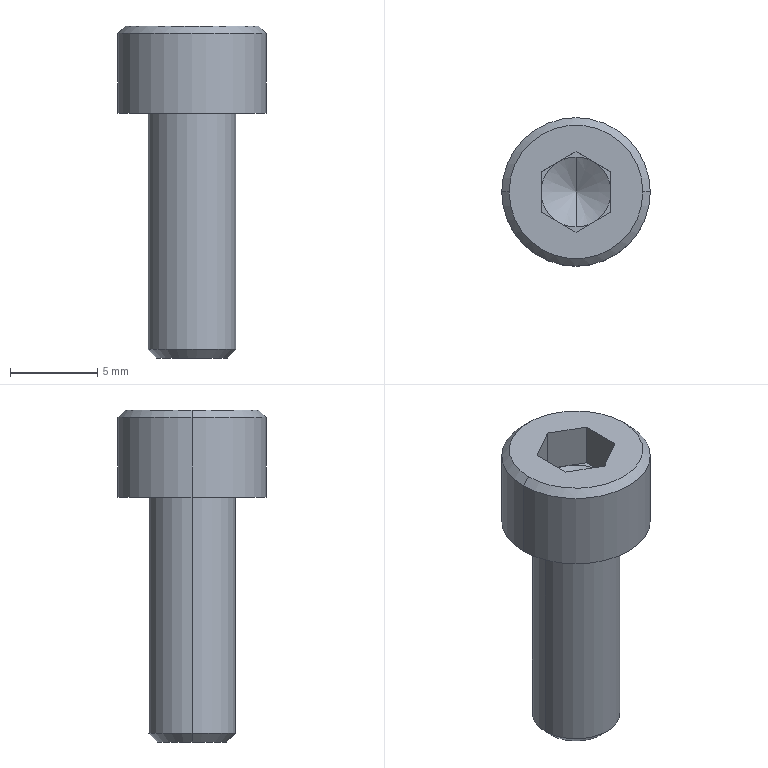Part | NX | features BREP 1 | 1 solid | 25 faces | box 8.5 x 8.5 x 19 mm | volume 515.039 mm3 | plane 15 | cone 6 | cylinder 4 | commonest cylinder face diameters 5 x2 8.5 x2
STEP:
#1=CARTESIAN_POINT('',(0.,-2.,2.5));
#2=VERTEX_POINT('',#1);
#3=CARTESIAN_POINT('',(0.,0.,1.345));
#4=VERTEX_POINT('',#3);
#5=CARTESIAN_POINT('',(0.,0.,1.345));
#6=DIRECTION('',(0.,-0.866,0.5));
#7=VECTOR('',#6,1000.);
#8=LINE('',#5,#7);
#9=EDGE_CURVE('',#2,#4,#8,.F.);
#10=ORIENTED_EDGE('',*,*,#9,.T.);
#11=CARTESIAN_POINT('',(0.,2.,2.5));
#12=VERTEX_POINT('',#11);
#13=CARTESIAN_POINT('',(0.,0.,1.345));
#14=DIRECTION('',(0.,0.866,0.5));
#15=VECTOR('',#14,1000.);
#16=LINE('',#13,#15);
#17=EDGE_CURVE('',#12,#4,#16,.F.);
#18=ORIENTED_EDGE('',*,*,#17,.F.);
#19=CARTESIAN_POINT('',(-1.,1.732,2.5));
#20=VERTEX_POINT('',#19);
#21=CARTESIAN_POINT('',(0.,0.,2.5));
#22=DIRECTION('',(0.,0.,1.));
#23=DIRECTION('',(0.,-1.,0.));
#24=AXIS2_PLACEMENT_3D('',#21,#22,#23);
#25=CIRCLE('',#24,2.);
#26=EDGE_CURVE('',#12,#20,#25,.T.);
#27=ORIENTED_EDGE('',*,*,#26,.T.);
#28=CARTESIAN_POINT('',(-2.,0.,2.5));
#29=VERTEX_POINT('',#28);
#30=CARTESIAN_POINT('',(0.,0.,2.5));
#31=DIRECTION('',(0.,0.,1.));
#32=DIRECTION('',(0.,-1.,0.));
#33=AXIS2_PLACEMENT_3D('',#30,#31,#32);
#34=CIRCLE('',#33,2.);
#35=EDGE_CURVE('',#20,#29,#34,.T.);
#36=ORIENTED_EDGE('',*,*,#35,.T.);
#37=CARTESIAN_POINT('',(-1.,-1.732,2.5));
#38=VERTEX_POINT('',#37);
#39=CARTESIAN_POINT('',(0.,0.,2.5));
#40=DIRECTION('',(0.,0.,1.));
#41=DIRECTION('',(0.,-1.,0.));
#42=AXIS2_PLACEMENT_3D('',#39,#40,#41);
#43=CIRCLE('',#42,2.);
#44=EDGE_CURVE('',#29,#38,#43,.T.);
#45=ORIENTED_EDGE('',*,*,#44,.T.);
#46=CARTESIAN_POINT('',(0.,0.,2.5));
#47=DIRECTION('',(0.,0.,1.));
#48=DIRECTION('',(0.,-1.,0.));
#49=AXIS2_PLACEMENT_3D('',#46,#47,#48);
#50=CIRCLE('',#49,2.);
#51=EDGE_CURVE('',#38,#2,#50,.T.);
#52=ORIENTED_EDGE('',*,*,#51,.T.);
#53=EDGE_LOOP('',(#10,#18,#27,#36,#45,#52));
#54=FACE_BOUND('',#53,.T.);
#55=CARTESIAN_POINT('',(0.,0.,1001.345));
#56=DIRECTION('',(0.,0.,1.));
#57=DIRECTION('',(0.,1.,0.));
#58=AXIS2_PLACEMENT_3D('',#55,#56,#57);
#59=CONICAL_SURFACE('',#58,1732.051,1.047);
#60=ADVANCED_FACE('',(#54),#59,.F.);
#61=CARTESIAN_POINT('',(4.25,0.,0.));
#62=VERTEX_POINT('',#61);
#63=CARTESIAN_POINT('',(-4.25,0.,0.));
#64=VERTEX_POINT('',#63);
#65=CARTESIAN_POINT('',(0.,0.,0.));
#66=DIRECTION('',(0.,0.,1.));
#67=DIRECTION('',(1.,0.,0.));
#68=AXIS2_PLACEMENT_3D('',#65,#66,#67);
#69=CIRCLE('',#68,4.25);
#70=EDGE_CURVE('',#62,#64,#69,.T.);
#71=ORIENTED_EDGE('',*,*,#70,.T.);
#72=CARTESIAN_POINT('',(-4.25,0.,4.575));
#73=VERTEX_POINT('',#72);
#74=CARTESIAN_POINT('',(-4.25,0.,0.));
#75=DIRECTION('',(0.,0.,1.));
#76=VECTOR('',#75,1000.);
#77=LINE('',#74,#76);
#78=EDGE_CURVE('',#64,#73,#77,.T.);
#79=ORIENTED_EDGE('',*,*,#78,.T.);
#80=CARTESIAN_POINT('',(4.25,0.,4.575));
#81=VERTEX_POINT('',#80);
#82=CARTESIAN_POINT('',(0.,0.,4.575));
#83=DIRECTION('',(0.,0.,1.));
#84=DIRECTION('',(1.,0.,0.));
#85=AXIS2_PLACEMENT_3D('',#82,#83,#84);
#86=CIRCLE('',#85,4.25);
#87=EDGE_CURVE('',#81,#73,#86,.T.);
#88=ORIENTED_EDGE('',*,*,#87,.F.);
#89=CARTESIAN_POINT('',(4.25,0.,0.));
#90=DIRECTION('',(0.,0.,1.));
#91=VECTOR('',#90,1000.);
#92=LINE('',#89,#91);
#93=EDGE_CURVE('',#62,#81,#92,.T.);
#94=ORIENTED_EDGE('',*,*,#93,.F.);
#95=EDGE_LOOP('',(#71,#79,#88,#94));
#96=FACE_BOUND('',#95,.T.);
#97=CARTESIAN_POINT('',(0.,0.,0.));
#98=DIRECTION('',(0.,0.,1.));
#99=DIRECTION('',(-1.,0.,0.));
#100=AXIS2_PLACEMENT_3D('',#97,#98,#99);
#101=CYLINDRICAL_SURFACE('',#100,4.25);
#102=ADVANCED_FACE('',(#96),#101,.T.);
#103=CARTESIAN_POINT('',(3.825,0.,5.));
#104=VERTEX_POINT('',#103);
#105=CARTESIAN_POINT('',(-3.825,0.,5.));
#106=VERTEX_POINT('',#105);
#107=CARTESIAN_POINT('',(0.,0.,5.));
#108=DIRECTION('',(0.,0.,1.));
#109=DIRECTION('',(1.,0.,0.));
#110=AXIS2_PLACEMENT_3D('',#107,#108,#109);
#111=CIRCLE('',#110,3.825);
#112=EDGE_CURVE('',#104,#106,#111,.T.);
#113=ORIENTED_EDGE('',*,*,#112,.F.);
#114=CARTESIAN_POINT('',(4.25,0.,4.575));
#115=DIRECTION('',(0.7071,0.,-0.7071));
#116=VECTOR('',#115,1000.);
#117=LINE('',#114,#116);
#118=EDGE_CURVE('',#81,#104,#117,.F.);
#119=ORIENTED_EDGE('',*,*,#118,.F.);
#120=ORIENTED_EDGE('',*,*,#87,.T.);
#121=CARTESIAN_POINT('',(-4.25,0.,4.575));
#122=DIRECTION('',(-0.7071,0.,-0.7071));
#123=VECTOR('',#122,1000.);
#124=LINE('',#121,#123);
#125=EDGE_CURVE('',#73,#106,#124,.F.);
#126=ORIENTED_EDGE('',*,*,#125,.T.);
#127=EDGE_LOOP('',(#113,#119,#120,#126));
#128=FACE_BOUND('',#127,.T.);
#129=CARTESIAN_POINT('',(0.,0.,4.575));
#130=DIRECTION('',(0.,0.,-1.));
#131=DIRECTION('',(1.,0.,0.));
#132=AXIS2_PLACEMENT_3D('',#129,#130,#131);
#133=CONICAL_SURFACE('',#132,4.25,0.7854);
#134=ADVANCED_FACE('',(#128),#133,.T.);
#135=CARTESIAN_POINT('',(2.01,0.,-14.));
#136=VERTEX_POINT('',#135);
#137=CARTESIAN_POINT('',(-2.01,0.,-14.));
#138=VERTEX_POINT('',#137);
#139=CARTESIAN_POINT('',(0.,0.,-14.));
#140=DIRECTION('',(0.,0.,1.));
#141=DIRECTION('',(1.,0.,0.));
#142=AXIS2_PLACEMENT_3D('',#139,#140,#141);
#143=CIRCLE('',#142,2.01);
#144=EDGE_CURVE('',#136,#138,#143,.T.);
#145=ORIENTED_EDGE('',*,*,#144,.T.);
#146=CARTESIAN_POINT('',(-2.5,0.,-13.509));
#147=VERTEX_POINT('',#146);
#148=CARTESIAN_POINT('',(-2.01,0.,-14.));
#149=DIRECTION('',(-0.7071,0.,0.7071));
#150=VECTOR('',#149,1000.);
#151=LINE('',#148,#150);
#152=EDGE_CURVE('',#138,#147,#151,.T.);
#153=ORIENTED_EDGE('',*,*,#152,.T.);
#154=CARTESIAN_POINT('',(2.5,0.,-13.509));
#155=VERTEX_POINT('',#154);
#156=CARTESIAN_POINT('',(0.,0.,-13.509));
#157=DIRECTION('',(0.,0.,1.));
#158=DIRECTION('',(1.,0.,0.));
#159=AXIS2_PLACEMENT_3D('',#156,#157,#158);
#160=CIRCLE('',#159,2.5);
#161=EDGE_CURVE('',#155,#147,#160,.T.);
#162=ORIENTED_EDGE('',*,*,#161,.F.);
#163=CARTESIAN_POINT('',(2.01,0.,-14.));
#164=DIRECTION('',(0.7071,0.,0.7071));
#165=VECTOR('',#164,1000.);
#166=LINE('',#163,#165);
#167=EDGE_CURVE('',#136,#155,#166,.T.);
#168=ORIENTED_EDGE('',*,*,#167,.F.);
#169=EDGE_LOOP('',(#145,#153,#162,#168));
#170=FACE_BOUND('',#169,.T.);
#171=CARTESIAN_POINT('',(0.,0.,-14.));
#172=DIRECTION('',(0.,0.,1.));
#173=DIRECTION('',(-1.,0.,0.));
#174=AXIS2_PLACEMENT_3D('',#171,#172,#173);
#175=CONICAL_SURFACE('',#174,2.01,0.7854);
#176=ADVANCED_FACE('',(#170),#175,.T.);
#177=ORIENTED_EDGE('',*,*,#161,.T.);
#178=CARTESIAN_POINT('',(-2.5,0.,0.));
#179=VERTEX_POINT('',#178);
#180=CARTESIAN_POINT('',(-2.5,0.,-14.));
#181=DIRECTION('',(0.,0.,1.));
#182=VECTOR('',#181,1000.);
#183=LINE('',#180,#182);
#184=EDGE_CURVE('',#147,#179,#183,.T.);
#185=ORIENTED_EDGE('',*,*,#184,.T.);
#186=CARTESIAN_POINT('',(2.5,0.,0.));
#187=VERTEX_POINT('',#186);
#188=CARTESIAN_POINT('',(0.,0.,0.));
#189=DIRECTION('',(0.,0.,1.));
#190=DIRECTION('',(1.,0.,0.));
#191=AXIS2_PLACEMENT_3D('',#188,#189,#190);
#192=CIRCLE('',#191,2.5);
#193=EDGE_CURVE('',#187,#179,#192,.T.);
#194=ORIENTED_EDGE('',*,*,#193,.F.);
#195=CARTESIAN_POINT('',(2.5,0.,-14.));
#196=DIRECTION('',(0.,0.,1.));
#197=VECTOR('',#196,1000.);
#198=LINE('',#195,#197);
#199=EDGE_CURVE('',#155,#187,#198,.T.);
#200=ORIENTED_EDGE('',*,*,#199,.F.);
#201=EDGE_LOOP('',(#177,#185,#194,#200));
#202=FACE_BOUND('',#201,.T.);
#203=CARTESIAN_POINT('',(0.,0.,-14.));
#204=DIRECTION('',(0.,0.,1.));
#205=DIRECTION('',(-1.,0.,0.));
#206=AXIS2_PLACEMENT_3D('',#203,#204,#205);
#207=CYLINDRICAL_SURFACE('',#206,2.5);
#208=ADVANCED_FACE('',(#202),#207,.T.);
#209=CARTESIAN_POINT('',(1.,-1.732,2.5));
#210=VERTEX_POINT('',#209);
#211=CARTESIAN_POINT('',(2.,0.,2.5));
#212=VERTEX_POINT('',#211);
#213=CARTESIAN_POINT('',(0.,0.,2.5));
#214=DIRECTION('',(0.,0.,1.));
#215=DIRECTION('',(0.,-1.,0.));
#216=AXIS2_PLACEMENT_3D('',#213,#214,#215);
#217=CIRCLE('',#216,2.);
#218=EDGE_CURVE('',#210,#212,#217,.T.);
#219=ORIENTED_EDGE('',*,*,#218,.F.);
#220=CARTESIAN_POINT('',(2.,-1.155,2.5));
#221=VERTEX_POINT('',#220);
#222=CARTESIAN_POINT('',(0.,-2.309,2.5));
#223=DIRECTION('',(0.866,0.5,0.));
#224=VECTOR('',#223,1000.);
#225=LINE('',#222,#224);
#226=EDGE_CURVE('',#210,#221,#225,.T.);
#227=ORIENTED_EDGE('',*,*,#226,.T.);
#228=CARTESIAN_POINT('',(2.,-1.155,2.5));
#229=DIRECTION('',(0.,1.,0.));
#230=VECTOR('',#229,1000.);
#231=LINE('',#228,#230);
#232=EDGE_CURVE('',#221,#212,#231,.T.);
#233=ORIENTED_EDGE('',*,*,#232,.T.);
#234=EDGE_LOOP('',(#219,#227,#233));
#235=FACE_BOUND('',#234,.T.);
#236=CARTESIAN_POINT('',(0.,0.,2.5));
#237=DIRECTION('',(0.,0.,1.));
#238=DIRECTION('',(-1.,0.,0.));
#239=AXIS2_PLACEMENT_3D('',#236,#237,#238);
#240=PLANE('',#239);
#241=ADVANCED_FACE('',(#235),#240,.T.);
#242=CARTESIAN_POINT('',(1.,1.732,2.5));
#243=VERTEX_POINT('',#242);
#244=CARTESIAN_POINT('',(0.,0.,2.5));
#245=DIRECTION('',(0.,0.,1.));
#246=DIRECTION('',(0.,-1.,0.));
#247=AXIS2_PLACEMENT_3D('',#244,#245,#246);
#248=CIRCLE('',#247,2.);
#249=EDGE_CURVE('',#212,#243,#248,.T.);
#250=ORIENTED_EDGE('',*,*,#249,.F.);
#251=CARTESIAN_POINT('',(2.,1.155,2.5));
#252=VERTEX_POINT('',#251);
#253=CARTESIAN_POINT('',(2.,-1.155,2.5));
#254=DIRECTION('',(0.,1.,0.));
#255=VECTOR('',#254,1000.);
#256=LINE('',#253,#255);
#257=EDGE_CURVE('',#212,#252,#256,.T.);
#258=ORIENTED_EDGE('',*,*,#257,.T.);
#259=CARTESIAN_POINT('',(2.,1.155,2.5));
#260=DIRECTION('',(-0.866,0.5,0.));
#261=VECTOR('',#260,1000.);
#262=LINE('',#259,#261);
#263=EDGE_CURVE('',#252,#243,#262,.T.);
#264=ORIENTED_EDGE('',*,*,#263,.T.);
#265=EDGE_LOOP('',(#250,#258,#264));
#266=FACE_BOUND('',#265,.T.);
#267=CARTESIAN_POINT('',(0.,0.,2.5));
#268=DIRECTION('',(0.,0.,1.));
#269=DIRECTION('',(-1.,0.,0.));
#270=AXIS2_PLACEMENT_3D('',#267,#268,#269);
#271=PLANE('',#270);
#272=ADVANCED_FACE('',(#266),#271,.T.);
#273=CARTESIAN_POINT('',(0.,0.,2.5));
#274=DIRECTION('',(0.,0.,1.));
#275=DIRECTION('',(0.,-1.,0.));
#276=AXIS2_PLACEMENT_3D('',#273,#274,#275);
#277=CIRCLE('',#276,2.);
#278=EDGE_CURVE('',#243,#12,#277,.T.);
#279=ORIENTED_EDGE('',*,*,#278,.F.);
#280=CARTESIAN_POINT('',(0.,2.309,2.5));
#281=VERTEX_POINT('',#280);
#282=CARTESIAN_POINT('',(2.,1.155,2.5));
#283=DIRECTION('',(-0.866,0.5,0.));
#284=VECTOR('',#283,1000.);
#285=LINE('',#282,#284);
#286=EDGE_CURVE('',#243,#281,#285,.T.);
#287=ORIENTED_EDGE('',*,*,#286,.T.);
#288=CARTESIAN_POINT('',(0.,2.309,2.5));
#289=DIRECTION('',(-0.866,-0.5,0.));
#290=VECTOR('',#289,1000.);
#291=LINE('',#288,#290);
#292=EDGE_CURVE('',#281,#20,#291,.T.);
#293=ORIENTED_EDGE('',*,*,#292,.T.);
#294=ORIENTED_EDGE('',*,*,#26,.F.);
#295=EDGE_LOOP('',(#279,#287,#293,#294));
#296=FACE_BOUND('',#295,.T.);
#297=CARTESIAN_POINT('',(0.,0.,2.5));
#298=DIRECTION('',(0.,0.,1.));
#299=DIRECTION('',(-1.,0.,0.));
#300=AXIS2_PLACEMENT_3D('',#297,#298,#299);
#301=PLANE('',#300);
#302=ADVANCED_FACE('',(#296),#301,.T.);
#303=ORIENTED_EDGE('',*,*,#35,.F.);
#304=CARTESIAN_POINT('',(-2.,1.155,2.5));
#305=VERTEX_POINT('',#304);
#306=CARTESIAN_POINT('',(0.,2.309,2.5));
#307=DIRECTION('',(-0.866,-0.5,0.));
#308=VECTOR('',#307,1000.);
#309=LINE('',#306,#308);
#310=EDGE_CURVE('',#20,#305,#309,.T.);
#311=ORIENTED_EDGE('',*,*,#310,.T.);
#312=CARTESIAN_POINT('',(-2.,1.155,2.5));
#313=DIRECTION('',(0.,-1.,0.));
#314=VECTOR('',#313,1000.);
#315=LINE('',#312,#314);
#316=EDGE_CURVE('',#305,#29,#315,.T.);
#317=ORIENTED_EDGE('',*,*,#316,.T.);
#318=EDGE_LOOP('',(#303,#311,#317));
#319=FACE_BOUND('',#318,.T.);
#320=CARTESIAN_POINT('',(0.,0.,2.5));
#321=DIRECTION('',(0.,0.,1.));
#322=DIRECTION('',(-1.,0.,0.));
#323=AXIS2_PLACEMENT_3D('',#320,#321,#322);
#324=PLANE('',#323);
#325=ADVANCED_FACE('',(#319),#324,.T.);
#326=ORIENTED_EDGE('',*,*,#44,.F.);
#327=CARTESIAN_POINT('',(-2.,-1.155,2.5));
#328=VERTEX_POINT('',#327);
#329=CARTESIAN_POINT('',(-2.,1.155,2.5));
#330=DIRECTION('',(0.,-1.,0.));
#331=VECTOR('',#330,1000.);
#332=LINE('',#329,#331);
#333=EDGE_CURVE('',#29,#328,#332,.T.);
#334=ORIENTED_EDGE('',*,*,#333,.T.);
#335=CARTESIAN_POINT('',(-2.,-1.155,2.5));
#336=DIRECTION('',(0.866,-0.5,0.));
#337=VECTOR('',#336,1000.);
#338=LINE('',#335,#337);
#339=EDGE_CURVE('',#328,#38,#338,.T.);
#340=ORIENTED_EDGE('',*,*,#339,.T.);
#341=EDGE_LOOP('',(#326,#334,#340));
#342=FACE_BOUND('',#341,.T.);
#343=CARTESIAN_POINT('',(0.,0.,2.5));
#344=DIRECTION('',(0.,0.,1.));
#345=DIRECTION('',(-1.,0.,0.));
#346=AXIS2_PLACEMENT_3D('',#343,#344,#345);
#347=PLANE('',#346);
#348=ADVANCED_FACE('',(#342),#347,.T.);
#349=ORIENTED_EDGE('',*,*,#184,.F.);
#350=CARTESIAN_POINT('',(0.,0.,-13.509));
#351=DIRECTION('',(0.,0.,1.));
#352=DIRECTION('',(1.,0.,0.));
#353=AXIS2_PLACEMENT_3D('',#350,#351,#352);
#354=CIRCLE('',#353,2.5);
#355=EDGE_CURVE('',#147,#155,#354,.T.);
#356=ORIENTED_EDGE('',*,*,#355,.T.);
#357=ORIENTED_EDGE('',*,*,#199,.T.);
#358=CARTESIAN_POINT('',(0.,0.,0.));
#359=DIRECTION('',(0.,0.,1.));
#360=DIRECTION('',(1.,0.,0.));
#361=AXIS2_PLACEMENT_3D('',#358,#359,#360);
#362=CIRCLE('',#361,2.5);
#363=EDGE_CURVE('',#179,#187,#362,.T.);
#364=ORIENTED_EDGE('',*,*,#363,.F.);
#365=EDGE_LOOP('',(#349,#356,#357,#364));
#366=FACE_BOUND('',#365,.T.);
#367=CARTESIAN_POINT('',(0.,0.,-14.));
#368=DIRECTION('',(0.,0.,1.));
#369=DIRECTION('',(-1.,0.,0.));
#370=AXIS2_PLACEMENT_3D('',#367,#368,#369);
#371=CYLINDRICAL_SURFACE('',#370,2.5);
#372=ADVANCED_FACE('',(#366),#371,.T.);
#373=ORIENTED_EDGE('',*,*,#152,.F.);
#374=CARTESIAN_POINT('',(0.,0.,-14.));
#375=DIRECTION('',(0.,0.,1.));
#376=DIRECTION('',(1.,0.,0.));
#377=AXIS2_PLACEMENT_3D('',#374,#375,#376);
#378=CIRCLE('',#377,2.01);
#379=EDGE_CURVE('',#138,#136,#378,.T.);
#380=ORIENTED_EDGE('',*,*,#379,.T.);
#381=ORIENTED_EDGE('',*,*,#167,.T.);
#382=ORIENTED_EDGE('',*,*,#355,.F.);
#383=EDGE_LOOP('',(#373,#380,#381,#382));
#384=FACE_BOUND('',#383,.T.);
#385=CARTESIAN_POINT('',(0.,0.,-14.));
#386=DIRECTION('',(0.,0.,1.));
#387=DIRECTION('',(-1.,0.,0.));
#388=AXIS2_PLACEMENT_3D('',#385,#386,#387);
#389=CONICAL_SURFACE('',#388,2.01,0.7854);
#390=ADVANCED_FACE('',(#384),#389,.T.);
#391=ORIENTED_EDGE('',*,*,#144,.F.);
#392=ORIENTED_EDGE('',*,*,#379,.F.);
#393=EDGE_LOOP('',(#391,#392));
#394=FACE_BOUND('',#393,.T.);
#395=CARTESIAN_POINT('',(0.,2.01,-14.));
#396=DIRECTION('',(0.,0.,1.));
#397=DIRECTION('',(-1.,0.,0.));
#398=AXIS2_PLACEMENT_3D('',#395,#396,#397);
#399=PLANE('',#398);
#400=ADVANCED_FACE('',(#394),#399,.F.);
#401=CARTESIAN_POINT('',(0.,-2.309,5.));
#402=VERTEX_POINT('',#401);
#403=CARTESIAN_POINT('',(2.,-1.155,5.));
#404=VERTEX_POINT('',#403);
#405=CARTESIAN_POINT('',(0.,-2.309,5.));
#406=DIRECTION('',(0.866,0.5,0.));
#407=VECTOR('',#406,1000.);
#408=LINE('',#405,#407);
#409=EDGE_CURVE('',#402,#404,#408,.T.);
#410=ORIENTED_EDGE('',*,*,#409,.F.);
#411=CARTESIAN_POINT('',(-2.,-1.155,5.));
#412=VERTEX_POINT('',#411);
#413=CARTESIAN_POINT('',(-2.,-1.155,5.));
#414=DIRECTION('',(0.866,-0.5,0.));
#415=VECTOR('',#414,1000.);
#416=LINE('',#413,#415);
#417=EDGE_CURVE('',#412,#402,#416,.T.);
#418=ORIENTED_EDGE('',*,*,#417,.F.);
#419=CARTESIAN_POINT('',(-2.,1.155,5.));
#420=VERTEX_POINT('',#419);
#421=CARTESIAN_POINT('',(-2.,1.155,5.));
#422=DIRECTION('',(0.,-1.,0.));
#423=VECTOR('',#422,1000.);
#424=LINE('',#421,#423);
#425=EDGE_CURVE('',#420,#412,#424,.T.);
#426=ORIENTED_EDGE('',*,*,#425,.F.);
#427=CARTESIAN_POINT('',(0.,2.309,5.));
#428=VERTEX_POINT('',#427);
#429=CARTESIAN_POINT('',(0.,2.309,5.));
#430=DIRECTION('',(-0.866,-0.5,0.));
#431=VECTOR('',#430,1000.);
#432=LINE('',#429,#431);
#433=EDGE_CURVE('',#428,#420,#432,.T.);
#434=ORIENTED_EDGE('',*,*,#433,.F.);
#435=CARTESIAN_POINT('',(2.,1.155,5.));
#436=VERTEX_POINT('',#435);
#437=CARTESIAN_POINT('',(2.,1.155,5.));
#438=DIRECTION('',(-0.866,0.5,0.));
#439=VECTOR('',#438,1000.);
#440=LINE('',#437,#439);
#441=EDGE_CURVE('',#436,#428,#440,.T.);
#442=ORIENTED_EDGE('',*,*,#441,.F.);
#443=CARTESIAN_POINT('',(2.,-1.155,5.));
#444=DIRECTION('',(0.,1.,0.));
#445=VECTOR('',#444,1000.);
#446=LINE('',#443,#445);
#447=EDGE_CURVE('',#404,#436,#446,.T.);
#448=ORIENTED_EDGE('',*,*,#447,.F.);
#449=EDGE_LOOP('',(#410,#418,#426,#434,#442,#448));
#450=FACE_BOUND('',#449,.T.);
#451=CARTESIAN_POINT('',(0.,0.,5.));
#452=DIRECTION('',(0.,0.,1.));
#453=DIRECTION('',(1.,0.,0.));
#454=AXIS2_PLACEMENT_3D('',#451,#452,#453);
#455=CIRCLE('',#454,3.825);
#456=EDGE_CURVE('',#106,#104,#455,.T.);
#457=ORIENTED_EDGE('',*,*,#456,.T.);
#458=ORIENTED_EDGE('',*,*,#112,.T.);
#459=EDGE_LOOP('',(#457,#458));
#460=FACE_BOUND('',#459,.T.);
#461=CARTESIAN_POINT('',(0.,0.,5.));
#462=DIRECTION('',(0.,0.,-1.));
#463=DIRECTION('',(1.,0.,0.));
#464=AXIS2_PLACEMENT_3D('',#461,#462,#463);
#465=PLANE('',#464);
#466=ADVANCED_FACE('',(#450,#460),#465,.F.);
#467=ORIENTED_EDGE('',*,*,#118,.T.);
#468=ORIENTED_EDGE('',*,*,#456,.F.);
#469=ORIENTED_EDGE('',*,*,#125,.F.);
#470=CARTESIAN_POINT('',(0.,0.,4.575));
#471=DIRECTION('',(0.,0.,1.));
#472=DIRECTION('',(1.,0.,0.));
#473=AXIS2_PLACEMENT_3D('',#470,#471,#472);
#474=CIRCLE('',#473,4.25);
#475=EDGE_CURVE('',#73,#81,#474,.T.);
#476=ORIENTED_EDGE('',*,*,#475,.T.);
#477=EDGE_LOOP('',(#467,#468,#469,#476));
#478=FACE_BOUND('',#477,.T.);
#479=CARTESIAN_POINT('',(0.,0.,4.575));
#480=DIRECTION('',(0.,0.,-1.));
#481=DIRECTION('',(1.,0.,0.));
#482=AXIS2_PLACEMENT_3D('',#479,#480,#481);
#483=CONICAL_SURFACE('',#482,4.25,0.7854);
#484=ADVANCED_FACE('',(#478),#483,.T.);
#485=ORIENTED_EDGE('',*,*,#78,.F.);
#486=CARTESIAN_POINT('',(0.,0.,0.));
#487=DIRECTION('',(0.,0.,1.));
#488=DIRECTION('',(1.,0.,0.));
#489=AXIS2_PLACEMENT_3D('',#486,#487,#488);
#490=CIRCLE('',#489,4.25);
#491=EDGE_CURVE('',#64,#62,#490,.T.);
#492=ORIENTED_EDGE('',*,*,#491,.T.);
#493=ORIENTED_EDGE('',*,*,#93,.T.);
#494=ORIENTED_EDGE('',*,*,#475,.F.);
#495=EDGE_LOOP('',(#485,#492,#493,#494));
#496=FACE_BOUND('',#495,.T.);
#497=CARTESIAN_POINT('',(0.,0.,0.));
#498=DIRECTION('',(0.,0.,1.));
#499=DIRECTION('',(-1.,0.,0.));
#500=AXIS2_PLACEMENT_3D('',#497,#498,#499);
#501=CYLINDRICAL_SURFACE('',#500,4.25);
#502=ADVANCED_FACE('',(#496),#501,.T.);
#503=ORIENTED_EDGE('',*,*,#193,.T.);
#504=ORIENTED_EDGE('',*,*,#363,.T.);
#505=EDGE_LOOP('',(#503,#504));
#506=FACE_BOUND('',#505,.T.);
#507=ORIENTED_EDGE('',*,*,#70,.F.);
#508=ORIENTED_EDGE('',*,*,#491,.F.);
#509=EDGE_LOOP('',(#507,#508));
#510=FACE_BOUND('',#509,.T.);
#511=CARTESIAN_POINT('',(0.,4.25,0.));
#512=DIRECTION('',(0.,0.,1.));
#513=DIRECTION('',(-1.,0.,0.));
#514=AXIS2_PLACEMENT_3D('',#511,#512,#513);
#515=PLANE('',#514);
#516=ADVANCED_FACE('',(#506,#510),#515,.F.);
#517=ORIENTED_EDGE('',*,*,#417,.T.);
#518=CARTESIAN_POINT('',(0.,-2.309,2.5));
#519=VERTEX_POINT('',#518);
#520=CARTESIAN_POINT('',(0.,-2.309,2.5));
#521=DIRECTION('',(0.,0.,1.));
#522=VECTOR('',#521,1000.);
#523=LINE('',#520,#522);
#524=EDGE_CURVE('',#519,#402,#523,.T.);
#525=ORIENTED_EDGE('',*,*,#524,.F.);
#526=CARTESIAN_POINT('',(-2.,-1.155,2.5));
#527=DIRECTION('',(0.866,-0.5,0.));
#528=VECTOR('',#527,1000.);
#529=LINE('',#526,#528);
#530=EDGE_CURVE('',#38,#519,#529,.T.);
#531=ORIENTED_EDGE('',*,*,#530,.F.);
#532=ORIENTED_EDGE('',*,*,#339,.F.);
#533=CARTESIAN_POINT('',(-2.,-1.155,2.5));
#534=DIRECTION('',(0.,0.,1.));
#535=VECTOR('',#534,1000.);
#536=LINE('',#533,#535);
#537=EDGE_CURVE('',#328,#412,#536,.T.);
#538=ORIENTED_EDGE('',*,*,#537,.T.);
#539=EDGE_LOOP('',(#517,#525,#531,#532,#538));
#540=FACE_BOUND('',#539,.T.);
#541=CARTESIAN_POINT('',(-2.,-1.155,2.5));
#542=DIRECTION('',(-0.5,-0.866,0.));
#543=DIRECTION('',(-0.866,0.5,0.));
#544=AXIS2_PLACEMENT_3D('',#541,#542,#543);
#545=PLANE('',#544);
#546=ADVANCED_FACE('',(#540),#545,.F.);
#547=ORIENTED_EDGE('',*,*,#425,.T.);
#548=ORIENTED_EDGE('',*,*,#537,.F.);
#549=ORIENTED_EDGE('',*,*,#333,.F.);
#550=ORIENTED_EDGE('',*,*,#316,.F.);
#551=CARTESIAN_POINT('',(-2.,1.155,2.5));
#552=DIRECTION('',(0.,0.,1.));
#553=VECTOR('',#552,1000.);
#554=LINE('',#551,#553);
#555=EDGE_CURVE('',#305,#420,#554,.T.);
#556=ORIENTED_EDGE('',*,*,#555,.T.);
#557=EDGE_LOOP('',(#547,#548,#549,#550,#556));
#558=FACE_BOUND('',#557,.T.);
#559=CARTESIAN_POINT('',(-2.,1.155,2.5));
#560=DIRECTION('',(-1.,0.,0.));
#561=DIRECTION('',(0.,0.,-1.));
#562=AXIS2_PLACEMENT_3D('',#559,#560,#561);
#563=PLANE('',#562);
#564=ADVANCED_FACE('',(#558),#563,.F.);
#565=ORIENTED_EDGE('',*,*,#433,.T.);
#566=ORIENTED_EDGE('',*,*,#555,.F.);
#567=ORIENTED_EDGE('',*,*,#310,.F.);
#568=ORIENTED_EDGE('',*,*,#292,.F.);
#569=CARTESIAN_POINT('',(0.,2.309,2.5));
#570=DIRECTION('',(0.,0.,1.));
#571=VECTOR('',#570,1000.);
#572=LINE('',#569,#571);
#573=EDGE_CURVE('',#281,#428,#572,.T.);
#574=ORIENTED_EDGE('',*,*,#573,.T.);
#575=EDGE_LOOP('',(#565,#566,#567,#568,#574));
#576=FACE_BOUND('',#575,.T.);
#577=CARTESIAN_POINT('',(0.,2.309,2.5));
#578=DIRECTION('',(-0.5,0.866,0.));
#579=DIRECTION('',(0.866,0.5,0.));
#580=AXIS2_PLACEMENT_3D('',#577,#578,#579);
#581=PLANE('',#580);
#582=ADVANCED_FACE('',(#576),#581,.F.);
#583=ORIENTED_EDGE('',*,*,#441,.T.);
#584=ORIENTED_EDGE('',*,*,#573,.F.);
#585=ORIENTED_EDGE('',*,*,#286,.F.);
#586=ORIENTED_EDGE('',*,*,#263,.F.);
#587=CARTESIAN_POINT('',(2.,1.155,2.5));
#588=DIRECTION('',(0.,0.,1.));
#589=VECTOR('',#588,1000.);
#590=LINE('',#587,#589);
#591=EDGE_CURVE('',#252,#436,#590,.T.);
#592=ORIENTED_EDGE('',*,*,#591,.T.);
#593=EDGE_LOOP('',(#583,#584,#585,#586,#592));
#594=FACE_BOUND('',#593,.T.);
#595=CARTESIAN_POINT('',(2.,1.155,2.5));
#596=DIRECTION('',(0.5,0.866,0.));
#597=DIRECTION('',(0.866,-0.5,0.));
#598=AXIS2_PLACEMENT_3D('',#595,#596,#597);
#599=PLANE('',#598);
#600=ADVANCED_FACE('',(#594),#599,.F.);
#601=ORIENTED_EDGE('',*,*,#447,.T.);
#602=ORIENTED_EDGE('',*,*,#591,.F.);
#603=ORIENTED_EDGE('',*,*,#257,.F.);
#604=ORIENTED_EDGE('',*,*,#232,.F.);
#605=CARTESIAN_POINT('',(2.,-1.155,2.5));
#606=DIRECTION('',(0.,0.,1.));
#607=VECTOR('',#606,1000.);
#608=LINE('',#605,#607);
#609=EDGE_CURVE('',#221,#404,#608,.T.);
#610=ORIENTED_EDGE('',*,*,#609,.T.);
#611=EDGE_LOOP('',(#601,#602,#603,#604,#610));
#612=FACE_BOUND('',#611,.T.);
#613=CARTESIAN_POINT('',(2.,-1.155,2.5));
#614=DIRECTION('',(1.,0.,0.));
#615=DIRECTION('',(0.,0.,1.));
#616=AXIS2_PLACEMENT_3D('',#613,#614,#615);
#617=PLANE('',#616);
#618=ADVANCED_FACE('',(#612),#617,.F.);
#619=ORIENTED_EDGE('',*,*,#409,.T.);
#620=ORIENTED_EDGE('',*,*,#609,.F.);
#621=ORIENTED_EDGE('',*,*,#226,.F.);
#622=CARTESIAN_POINT('',(0.,-2.309,2.5));
#623=DIRECTION('',(0.866,0.5,0.));
#624=VECTOR('',#623,1000.);
#625=LINE('',#622,#624);
#626=EDGE_CURVE('',#519,#210,#625,.T.);
#627=ORIENTED_EDGE('',*,*,#626,.F.);
#628=ORIENTED_EDGE('',*,*,#524,.T.);
#629=EDGE_LOOP('',(#619,#620,#621,#627,#628));
#630=FACE_BOUND('',#629,.T.);
#631=CARTESIAN_POINT('',(0.,-2.309,2.5));
#632=DIRECTION('',(0.5,-0.866,0.));
#633=DIRECTION('',(-0.866,-0.5,0.));
#634=AXIS2_PLACEMENT_3D('',#631,#632,#633);
#635=PLANE('',#634);
#636=ADVANCED_FACE('',(#630),#635,.F.);
#637=ORIENTED_EDGE('',*,*,#51,.F.);
#638=ORIENTED_EDGE('',*,*,#530,.T.);
#639=ORIENTED_EDGE('',*,*,#626,.T.);
#640=CARTESIAN_POINT('',(0.,0.,2.5));
#641=DIRECTION('',(0.,0.,1.));
#642=DIRECTION('',(0.,-1.,0.));
#643=AXIS2_PLACEMENT_3D('',#640,#641,#642);
#644=CIRCLE('',#643,2.);
#645=EDGE_CURVE('',#2,#210,#644,.T.);
#646=ORIENTED_EDGE('',*,*,#645,.F.);
#647=EDGE_LOOP('',(#637,#638,#639,#646));
#648=FACE_BOUND('',#647,.T.);
#649=CARTESIAN_POINT('',(0.,0.,2.5));
#650=DIRECTION('',(0.,0.,1.));
#651=DIRECTION('',(-1.,0.,0.));
#652=AXIS2_PLACEMENT_3D('',#649,#650,#651);
#653=PLANE('',#652);
#654=ADVANCED_FACE('',(#648),#653,.T.);
#655=ORIENTED_EDGE('',*,*,#17,.T.);
#656=ORIENTED_EDGE('',*,*,#9,.F.);
#657=ORIENTED_EDGE('',*,*,#645,.T.);
#658=ORIENTED_EDGE('',*,*,#218,.T.);
#659=ORIENTED_EDGE('',*,*,#249,.T.);
#660=ORIENTED_EDGE('',*,*,#278,.T.);
#661=EDGE_LOOP('',(#655,#656,#657,#658,#659,#660));
#662=FACE_BOUND('',#661,.T.);
#663=CARTESIAN_POINT('',(0.,0.,1001.345));
#664=DIRECTION('',(0.,0.,1.));
#665=DIRECTION('',(0.,1.,0.));
#666=AXIS2_PLACEMENT_3D('',#663,#664,#665);
#667=CONICAL_SURFACE('',#666,1732.051,1.047);
#668=ADVANCED_FACE('',(#662),#667,.F.);
#669=CLOSED_SHELL('',(#60,#102,#134,#176,#208,#241,#272,#302,#325,#348,#372,#390,#400,#466,#484,#502,#516,#546,#564,#582,#600,#618,#636,#654,#668));
#670=MANIFOLD_SOLID_BREP('',#669);
#671=(LENGTH_UNIT()NAMED_UNIT(*)SI_UNIT(.MILLI.,.METRE.));
#672=UNCERTAINTY_MEASURE_WITH_UNIT(LENGTH_MEASURE(0.00001),#671,'','');
#673=(NAMED_UNIT(*)PLANE_ANGLE_UNIT()SI_UNIT($,.RADIAN.));
#674=(NAMED_UNIT(*)SI_UNIT($,.STERADIAN.)SOLID_ANGLE_UNIT());
#675=(GEOMETRIC_REPRESENTATION_CONTEXT(3)GLOBAL_UNCERTAINTY_ASSIGNED_CONTEXT((#672))GLOBAL_UNIT_ASSIGNED_CONTEXT((#671,#673,#674))REPRESENTATION_CONTEXT('',''));
#676=ADVANCED_BREP_SHAPE_REPRESENTATION('',(#670),#675);